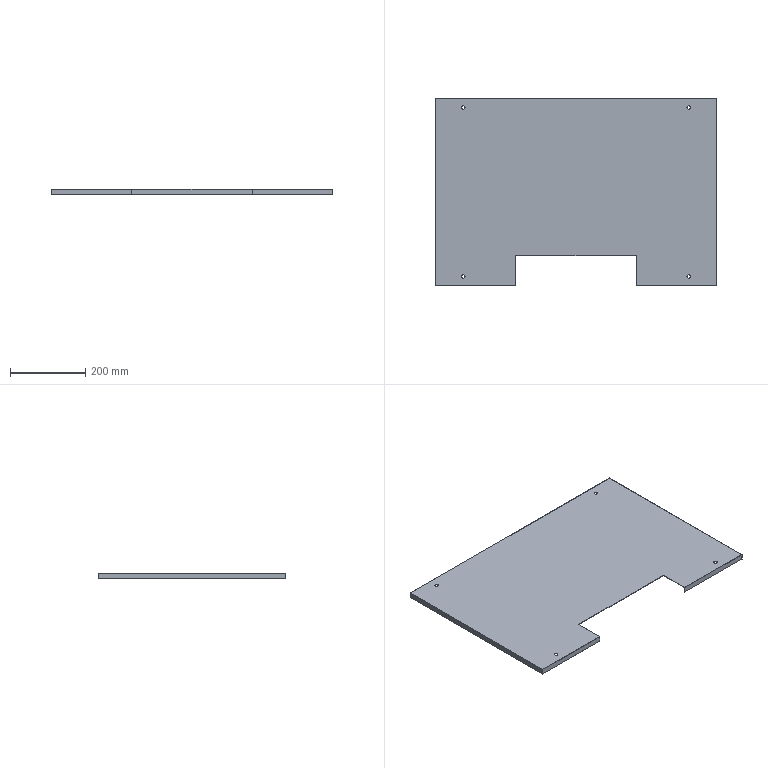Part | STEP file | 1 solid | 24 faces | box 750 x 500 x 15 mm | volume 567742 mm3 | plane 16 | cylinder 8 | commonest cylinder face diameters 9 x8